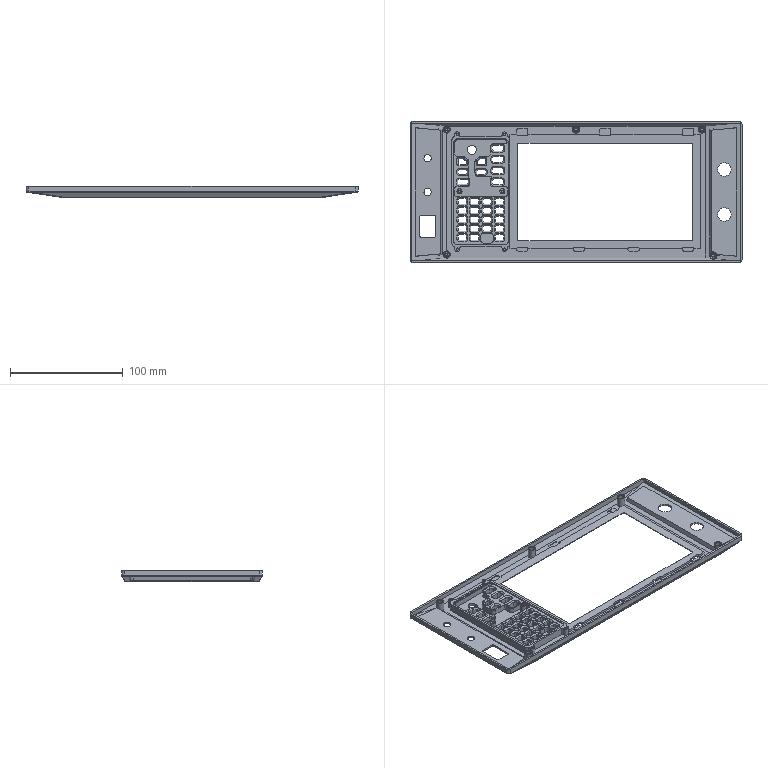Part | 1 solid | 1119 faces | box 295 x 125 x 10 mm | volume 58865 mm3 | plane 540 | cylinder 363 | cone 204 | spline 8 | sphere 4 | commonest cylinder face diameters 2.4 x160 3 x44 2 x32 4.4 x20 4.5 x18 6 x15